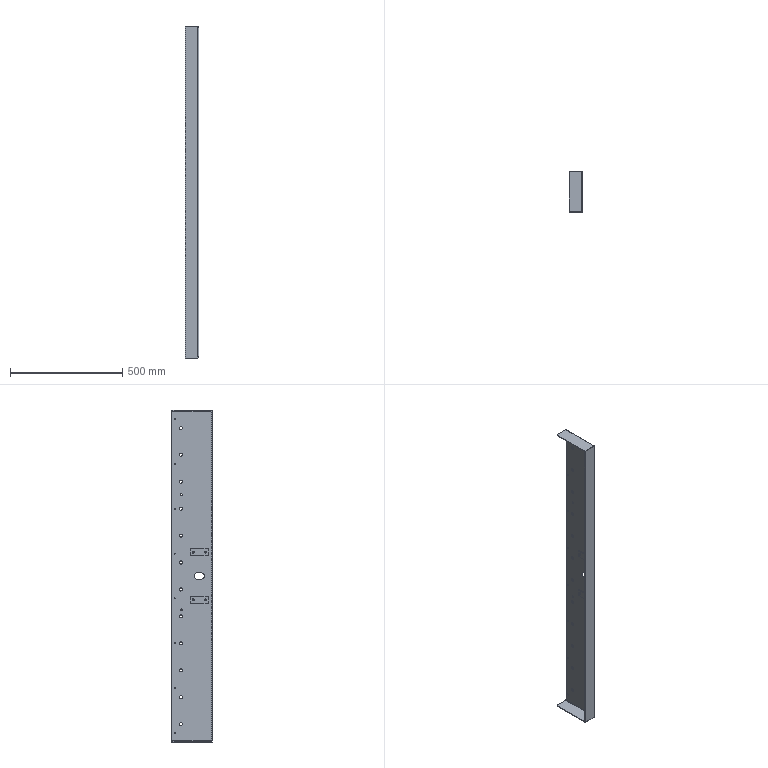Part | STEP file | 9-Body drive side_default<machined> | 3 solids | 148 faces | box 60 x 179.5 x 1480 mm | volume 1116104 mm3 | cylinder 82 | plane 66 | commonest cylinder face diameters 11 x44 5 x16 8.5 x8 6.8 x4 3 x3 9 x3